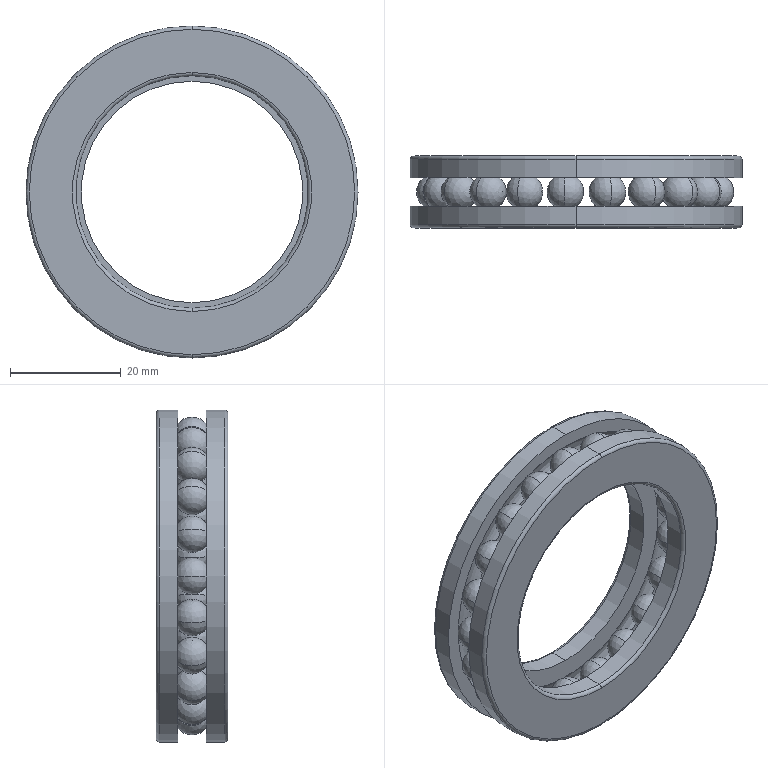Part | SolidWorks | features Revolution 3, CirPattern 1, Fillet 1 | 1 solid | 108 faces | box 60 x 13 x 60 mm | volume 14302 mm3 | torus 52 | sphere 42 | cylinder 8 | plane 6 | commonest cylinder face diameters 60 x4 40 x2 42 x2